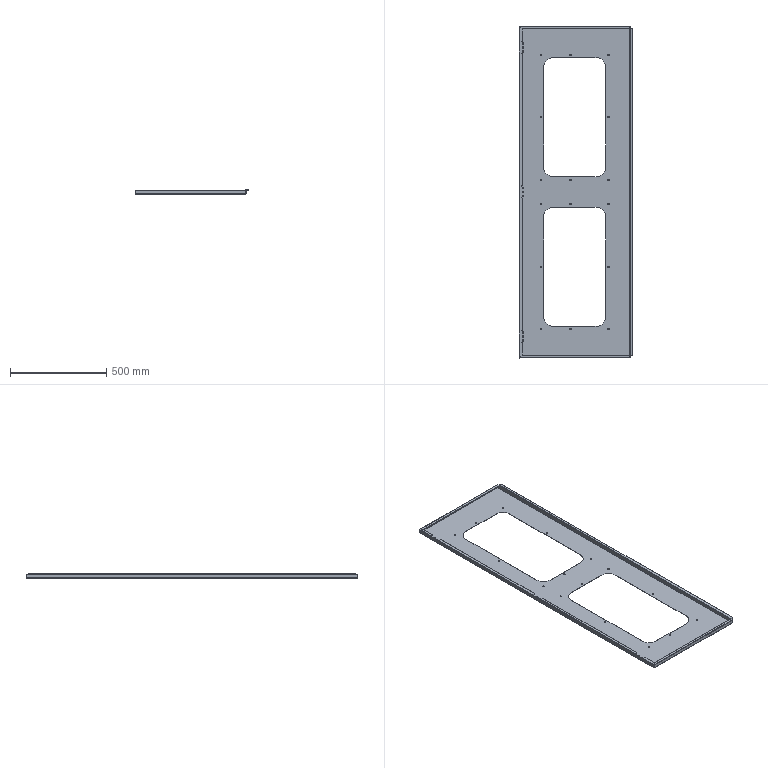Part | STEP file | Hinged door 1-left | 1 solid | 170 faces | box 587.5 x 1721 x 21.7 mm | volume 1104799 mm3 | cylinder 88 | plane 74 | spline 8 | commonest cylinder face diameters 7.5 x32 8.7 x18 0.4 x11 3.4 x11 10 x8 100 x8